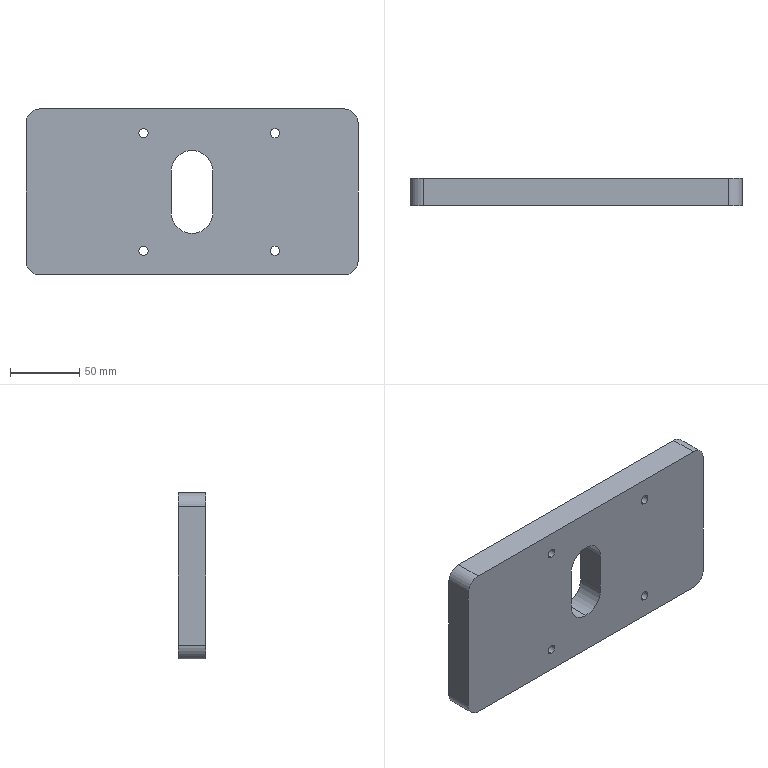Part | SolidWorks | features BaseBody 1 | 1 solid | 23 faces | box 240 x 20 x 120 mm | volume 539241 mm3 | cylinder 15 | plane 8 | commonest cylinder face diameters 6.8 x8 20 x4 30 x3
STEP:
#1=CARTESIAN_POINT('',(-35.,-10.,-45.9));
#2=VERTEX_POINT('',#1);
#3=CARTESIAN_POINT('',(-35.,-10.,-39.1));
#4=VERTEX_POINT('',#3);
#5=CARTESIAN_POINT('',(-35.,-10.,-42.5));
#6=DIRECTION('',(0.,1.,0.));
#7=DIRECTION('',(0.,0.,1.));
#8=AXIS2_PLACEMENT_3D('',#5,#6,#7);
#9=CIRCLE('',#8,3.4);
#10=EDGE_CURVE('',#2,#4,#9,.T.);
#11=ORIENTED_EDGE('',*,*,#10,.F.);
#12=CARTESIAN_POINT('',(-35.,10.,-45.9));
#13=VERTEX_POINT('',#12);
#14=CARTESIAN_POINT('',(-35.,10.,-45.9));
#15=DIRECTION('',(0.,1.,0.));
#16=VECTOR('',#15,1000.);
#17=LINE('',#14,#16);
#18=EDGE_CURVE('',#2,#13,#17,.T.);
#19=ORIENTED_EDGE('',*,*,#18,.T.);
#20=CARTESIAN_POINT('',(-35.,10.,-39.1));
#21=VERTEX_POINT('',#20);
#22=CARTESIAN_POINT('',(-35.,10.,-42.5));
#23=DIRECTION('',(0.,1.,0.));
#24=DIRECTION('',(0.,0.,1.));
#25=AXIS2_PLACEMENT_3D('',#22,#23,#24);
#26=CIRCLE('',#25,3.4);
#27=EDGE_CURVE('',#13,#21,#26,.T.);
#28=ORIENTED_EDGE('',*,*,#27,.T.);
#29=CARTESIAN_POINT('',(-35.,10.,-39.1));
#30=DIRECTION('',(0.,1.,0.));
#31=VECTOR('',#30,1000.);
#32=LINE('',#29,#31);
#33=EDGE_CURVE('',#4,#21,#32,.T.);
#34=ORIENTED_EDGE('',*,*,#33,.F.);
#35=EDGE_LOOP('',(#11,#19,#28,#34));
#36=FACE_OUTER_BOUND('',#35,.T.);
#37=CARTESIAN_POINT('',(-35.,10.,-42.5));
#38=DIRECTION('',(0.,1.,0.));
#39=DIRECTION('',(0.,0.,1.));
#40=AXIS2_PLACEMENT_3D('',#37,#38,#39);
#41=CYLINDRICAL_SURFACE('',#40,3.4);
#42=ADVANCED_FACE('',(#36),#41,.F.);
#43=CARTESIAN_POINT('',(60.,-10.,-45.9));
#44=VERTEX_POINT('',#43);
#45=CARTESIAN_POINT('',(60.,-10.,-39.1));
#46=VERTEX_POINT('',#45);
#47=CARTESIAN_POINT('',(60.,-10.,-42.5));
#48=DIRECTION('',(0.,1.,0.));
#49=DIRECTION('',(0.,0.,1.));
#50=AXIS2_PLACEMENT_3D('',#47,#48,#49);
#51=CIRCLE('',#50,3.4);
#52=EDGE_CURVE('',#44,#46,#51,.T.);
#53=ORIENTED_EDGE('',*,*,#52,.F.);
#54=CARTESIAN_POINT('',(60.,10.,-45.9));
#55=VERTEX_POINT('',#54);
#56=CARTESIAN_POINT('',(60.,10.,-45.9));
#57=DIRECTION('',(0.,1.,0.));
#58=VECTOR('',#57,1000.);
#59=LINE('',#56,#58);
#60=EDGE_CURVE('',#44,#55,#59,.T.);
#61=ORIENTED_EDGE('',*,*,#60,.T.);
#62=CARTESIAN_POINT('',(60.,10.,-39.1));
#63=VERTEX_POINT('',#62);
#64=CARTESIAN_POINT('',(60.,10.,-42.5));
#65=DIRECTION('',(0.,1.,0.));
#66=DIRECTION('',(0.,0.,1.));
#67=AXIS2_PLACEMENT_3D('',#64,#65,#66);
#68=CIRCLE('',#67,3.4);
#69=EDGE_CURVE('',#55,#63,#68,.T.);
#70=ORIENTED_EDGE('',*,*,#69,.T.);
#71=CARTESIAN_POINT('',(60.,10.,-39.1));
#72=DIRECTION('',(0.,1.,0.));
#73=VECTOR('',#72,1000.);
#74=LINE('',#71,#73);
#75=EDGE_CURVE('',#46,#63,#74,.T.);
#76=ORIENTED_EDGE('',*,*,#75,.F.);
#77=EDGE_LOOP('',(#53,#61,#70,#76));
#78=FACE_OUTER_BOUND('',#77,.T.);
#79=CARTESIAN_POINT('',(60.,10.,-42.5));
#80=DIRECTION('',(0.,1.,0.));
#81=DIRECTION('',(0.,0.,1.));
#82=AXIS2_PLACEMENT_3D('',#79,#80,#81);
#83=CYLINDRICAL_SURFACE('',#82,3.4);
#84=ADVANCED_FACE('',(#78),#83,.F.);
#85=CARTESIAN_POINT('',(60.,-10.,39.1));
#86=VERTEX_POINT('',#85);
#87=CARTESIAN_POINT('',(60.,-10.,45.9));
#88=VERTEX_POINT('',#87);
#89=CARTESIAN_POINT('',(60.,-10.,42.5));
#90=DIRECTION('',(0.,1.,0.));
#91=DIRECTION('',(0.,0.,1.));
#92=AXIS2_PLACEMENT_3D('',#89,#90,#91);
#93=CIRCLE('',#92,3.4);
#94=EDGE_CURVE('',#86,#88,#93,.T.);
#95=ORIENTED_EDGE('',*,*,#94,.F.);
#96=CARTESIAN_POINT('',(60.,10.,39.1));
#97=VERTEX_POINT('',#96);
#98=CARTESIAN_POINT('',(60.,10.,39.1));
#99=DIRECTION('',(0.,1.,0.));
#100=VECTOR('',#99,1000.);
#101=LINE('',#98,#100);
#102=EDGE_CURVE('',#86,#97,#101,.T.);
#103=ORIENTED_EDGE('',*,*,#102,.T.);
#104=CARTESIAN_POINT('',(60.,10.,45.9));
#105=VERTEX_POINT('',#104);
#106=CARTESIAN_POINT('',(60.,10.,42.5));
#107=DIRECTION('',(0.,1.,0.));
#108=DIRECTION('',(0.,0.,1.));
#109=AXIS2_PLACEMENT_3D('',#106,#107,#108);
#110=CIRCLE('',#109,3.4);
#111=EDGE_CURVE('',#97,#105,#110,.T.);
#112=ORIENTED_EDGE('',*,*,#111,.T.);
#113=CARTESIAN_POINT('',(60.,10.,45.9));
#114=DIRECTION('',(0.,1.,0.));
#115=VECTOR('',#114,1000.);
#116=LINE('',#113,#115);
#117=EDGE_CURVE('',#88,#105,#116,.T.);
#118=ORIENTED_EDGE('',*,*,#117,.F.);
#119=EDGE_LOOP('',(#95,#103,#112,#118));
#120=FACE_OUTER_BOUND('',#119,.T.);
#121=CARTESIAN_POINT('',(60.,10.,42.5));
#122=DIRECTION('',(0.,1.,0.));
#123=DIRECTION('',(0.,0.,1.));
#124=AXIS2_PLACEMENT_3D('',#121,#122,#123);
#125=CYLINDRICAL_SURFACE('',#124,3.4);
#126=ADVANCED_FACE('',(#120),#125,.F.);
#127=CARTESIAN_POINT('',(-35.,-10.,39.1));
#128=VERTEX_POINT('',#127);
#129=CARTESIAN_POINT('',(-35.,-10.,45.9));
#130=VERTEX_POINT('',#129);
#131=CARTESIAN_POINT('',(-35.,-10.,42.5));
#132=DIRECTION('',(0.,1.,0.));
#133=DIRECTION('',(0.,0.,1.));
#134=AXIS2_PLACEMENT_3D('',#131,#132,#133);
#135=CIRCLE('',#134,3.4);
#136=EDGE_CURVE('',#128,#130,#135,.T.);
#137=ORIENTED_EDGE('',*,*,#136,.F.);
#138=CARTESIAN_POINT('',(-35.,10.,39.1));
#139=VERTEX_POINT('',#138);
#140=CARTESIAN_POINT('',(-35.,10.,39.1));
#141=DIRECTION('',(0.,1.,0.));
#142=VECTOR('',#141,1000.);
#143=LINE('',#140,#142);
#144=EDGE_CURVE('',#128,#139,#143,.T.);
#145=ORIENTED_EDGE('',*,*,#144,.T.);
#146=CARTESIAN_POINT('',(-35.,10.,45.9));
#147=VERTEX_POINT('',#146);
#148=CARTESIAN_POINT('',(-35.,10.,42.5));
#149=DIRECTION('',(0.,1.,0.));
#150=DIRECTION('',(0.,0.,1.));
#151=AXIS2_PLACEMENT_3D('',#148,#149,#150);
#152=CIRCLE('',#151,3.4);
#153=EDGE_CURVE('',#139,#147,#152,.T.);
#154=ORIENTED_EDGE('',*,*,#153,.T.);
#155=CARTESIAN_POINT('',(-35.,10.,45.9));
#156=DIRECTION('',(0.,1.,0.));
#157=VECTOR('',#156,1000.);
#158=LINE('',#155,#157);
#159=EDGE_CURVE('',#130,#147,#158,.T.);
#160=ORIENTED_EDGE('',*,*,#159,.F.);
#161=EDGE_LOOP('',(#137,#145,#154,#160));
#162=FACE_OUTER_BOUND('',#161,.T.);
#163=CARTESIAN_POINT('',(-35.,10.,42.5));
#164=DIRECTION('',(0.,1.,0.));
#165=DIRECTION('',(0.,0.,1.));
#166=AXIS2_PLACEMENT_3D('',#163,#164,#165);
#167=CYLINDRICAL_SURFACE('',#166,3.4);
#168=ADVANCED_FACE('',(#162),#167,.F.);
#169=CARTESIAN_POINT('',(15.,10.,-15.));
#170=VERTEX_POINT('',#169);
#171=CARTESIAN_POINT('',(0.,10.,-30.));
#172=VERTEX_POINT('',#171);
#173=CARTESIAN_POINT('',(0.,10.,-15.));
#174=DIRECTION('',(0.,1.,0.));
#175=DIRECTION('',(0.,0.,1.));
#176=AXIS2_PLACEMENT_3D('',#173,#174,#175);
#177=CIRCLE('',#176,15.);
#178=EDGE_CURVE('',#170,#172,#177,.T.);
#179=ORIENTED_EDGE('',*,*,#178,.T.);
#180=CARTESIAN_POINT('',(0.,-10.,-30.));
#181=VERTEX_POINT('',#180);
#182=CARTESIAN_POINT('',(0.,10.,-30.));
#183=DIRECTION('',(0.,-1.,0.));
#184=VECTOR('',#183,1000.);
#185=LINE('',#182,#184);
#186=EDGE_CURVE('',#172,#181,#185,.T.);
#187=ORIENTED_EDGE('',*,*,#186,.T.);
#188=CARTESIAN_POINT('',(15.,-10.,-15.));
#189=VERTEX_POINT('',#188);
#190=CARTESIAN_POINT('',(0.,-10.,-15.));
#191=DIRECTION('',(0.,1.,0.));
#192=DIRECTION('',(0.,0.,1.));
#193=AXIS2_PLACEMENT_3D('',#190,#191,#192);
#194=CIRCLE('',#193,15.);
#195=EDGE_CURVE('',#189,#181,#194,.T.);
#196=ORIENTED_EDGE('',*,*,#195,.F.);
#197=CARTESIAN_POINT('',(15.,10.,-15.));
#198=DIRECTION('',(0.,-1.,0.));
#199=VECTOR('',#198,1000.);
#200=LINE('',#197,#199);
#201=EDGE_CURVE('',#170,#189,#200,.T.);
#202=ORIENTED_EDGE('',*,*,#201,.F.);
#203=EDGE_LOOP('',(#179,#187,#196,#202));
#204=FACE_OUTER_BOUND('',#203,.T.);
#205=CARTESIAN_POINT('',(0.,10.,-15.));
#206=DIRECTION('',(0.,-1.,0.));
#207=DIRECTION('',(0.,0.,-1.));
#208=AXIS2_PLACEMENT_3D('',#205,#206,#207);
#209=CYLINDRICAL_SURFACE('',#208,15.);
#210=ADVANCED_FACE('',(#204),#209,.F.);
#211=CARTESIAN_POINT('',(-35.,10.,-42.5));
#212=DIRECTION('',(0.,1.,0.));
#213=DIRECTION('',(0.,0.,1.));
#214=AXIS2_PLACEMENT_3D('',#211,#212,#213);
#215=CIRCLE('',#214,3.4);
#216=EDGE_CURVE('',#21,#13,#215,.T.);
#217=ORIENTED_EDGE('',*,*,#216,.F.);
#218=ORIENTED_EDGE('',*,*,#27,.F.);
#219=EDGE_LOOP('',(#217,#218));
#220=FACE_BOUND('',#219,.T.);
#221=CARTESIAN_POINT('',(60.,10.,-42.5));
#222=DIRECTION('',(0.,1.,0.));
#223=DIRECTION('',(0.,0.,1.));
#224=AXIS2_PLACEMENT_3D('',#221,#222,#223);
#225=CIRCLE('',#224,3.4);
#226=EDGE_CURVE('',#63,#55,#225,.T.);
#227=ORIENTED_EDGE('',*,*,#226,.F.);
#228=ORIENTED_EDGE('',*,*,#69,.F.);
#229=EDGE_LOOP('',(#227,#228));
#230=FACE_BOUND('',#229,.T.);
#231=CARTESIAN_POINT('',(60.,10.,42.5));
#232=DIRECTION('',(0.,1.,0.));
#233=DIRECTION('',(0.,0.,1.));
#234=AXIS2_PLACEMENT_3D('',#231,#232,#233);
#235=CIRCLE('',#234,3.4);
#236=EDGE_CURVE('',#105,#97,#235,.T.);
#237=ORIENTED_EDGE('',*,*,#236,.F.);
#238=ORIENTED_EDGE('',*,*,#111,.F.);
#239=EDGE_LOOP('',(#237,#238));
#240=FACE_BOUND('',#239,.T.);
#241=CARTESIAN_POINT('',(-35.,10.,42.5));
#242=DIRECTION('',(0.,1.,0.));
#243=DIRECTION('',(0.,0.,1.));
#244=AXIS2_PLACEMENT_3D('',#241,#242,#243);
#245=CIRCLE('',#244,3.4);
#246=EDGE_CURVE('',#147,#139,#245,.T.);
#247=ORIENTED_EDGE('',*,*,#246,.F.);
#248=ORIENTED_EDGE('',*,*,#153,.F.);
#249=EDGE_LOOP('',(#247,#248));
#250=FACE_BOUND('',#249,.T.);
#251=CARTESIAN_POINT('',(110.,10.,60.));
#252=VERTEX_POINT('',#251);
#253=CARTESIAN_POINT('',(120.,10.,50.));
#254=VERTEX_POINT('',#253);
#255=CARTESIAN_POINT('',(110.,10.,50.));
#256=DIRECTION('',(0.,1.,0.));
#257=DIRECTION('',(0.,0.,1.));
#258=AXIS2_PLACEMENT_3D('',#255,#256,#257);
#259=CIRCLE('',#258,10.);
#260=EDGE_CURVE('',#252,#254,#259,.T.);
#261=ORIENTED_EDGE('',*,*,#260,.T.);
#262=CARTESIAN_POINT('',(120.,10.,-50.));
#263=VERTEX_POINT('',#262);
#264=CARTESIAN_POINT('',(120.,10.,-50.));
#265=DIRECTION('',(0.,0.,-1.));
#266=VECTOR('',#265,1000.);
#267=LINE('',#264,#266);
#268=EDGE_CURVE('',#254,#263,#267,.T.);
#269=ORIENTED_EDGE('',*,*,#268,.T.);
#270=CARTESIAN_POINT('',(110.,10.,-60.));
#271=VERTEX_POINT('',#270);
#272=CARTESIAN_POINT('',(110.,10.,-50.));
#273=DIRECTION('',(0.,1.,0.));
#274=DIRECTION('',(0.,0.,-1.));
#275=AXIS2_PLACEMENT_3D('',#272,#273,#274);
#276=CIRCLE('',#275,10.);
#277=EDGE_CURVE('',#263,#271,#276,.T.);
#278=ORIENTED_EDGE('',*,*,#277,.T.);
#279=CARTESIAN_POINT('',(-110.,10.,-60.));
#280=VERTEX_POINT('',#279);
#281=CARTESIAN_POINT('',(-110.,10.,-60.));
#282=DIRECTION('',(-1.,0.,0.));
#283=VECTOR('',#282,1000.);
#284=LINE('',#281,#283);
#285=EDGE_CURVE('',#271,#280,#284,.T.);
#286=ORIENTED_EDGE('',*,*,#285,.T.);
#287=CARTESIAN_POINT('',(-120.,10.,-50.));
#288=VERTEX_POINT('',#287);
#289=CARTESIAN_POINT('',(-110.,10.,-50.));
#290=DIRECTION('',(0.,1.,0.));
#291=DIRECTION('',(0.,0.,1.));
#292=AXIS2_PLACEMENT_3D('',#289,#290,#291);
#293=CIRCLE('',#292,10.);
#294=EDGE_CURVE('',#280,#288,#293,.T.);
#295=ORIENTED_EDGE('',*,*,#294,.T.);
#296=CARTESIAN_POINT('',(-120.,10.,50.));
#297=VERTEX_POINT('',#296);
#298=CARTESIAN_POINT('',(-120.,10.,-50.));
#299=DIRECTION('',(0.,0.,1.));
#300=VECTOR('',#299,1000.);
#301=LINE('',#298,#300);
#302=EDGE_CURVE('',#288,#297,#301,.T.);
#303=ORIENTED_EDGE('',*,*,#302,.T.);
#304=CARTESIAN_POINT('',(-110.,10.,60.));
#305=VERTEX_POINT('',#304);
#306=CARTESIAN_POINT('',(-110.,10.,50.));
#307=DIRECTION('',(0.,1.,0.));
#308=DIRECTION('',(0.,0.,1.));
#309=AXIS2_PLACEMENT_3D('',#306,#307,#308);
#310=CIRCLE('',#309,10.);
#311=EDGE_CURVE('',#297,#305,#310,.T.);
#312=ORIENTED_EDGE('',*,*,#311,.T.);
#313=CARTESIAN_POINT('',(-110.,10.,60.));
#314=DIRECTION('',(1.,0.,0.));
#315=VECTOR('',#314,1000.);
#316=LINE('',#313,#315);
#317=EDGE_CURVE('',#305,#252,#316,.T.);
#318=ORIENTED_EDGE('',*,*,#317,.T.);
#319=EDGE_LOOP('',(#261,#269,#278,#286,#295,#303,#312,#318));
#320=FACE_OUTER_BOUND('',#319,.T.);
#321=CARTESIAN_POINT('',(-15.,10.,-15.));
#322=VERTEX_POINT('',#321);
#323=CARTESIAN_POINT('',(-15.,10.,15.));
#324=VERTEX_POINT('',#323);
#325=CARTESIAN_POINT('',(-15.,10.,-15.));
#326=DIRECTION('',(0.,0.,1.));
#327=VECTOR('',#326,1000.);
#328=LINE('',#325,#327);
#329=EDGE_CURVE('',#322,#324,#328,.T.);
#330=ORIENTED_EDGE('',*,*,#329,.F.);
#331=CARTESIAN_POINT('',(0.,10.,-15.));
#332=DIRECTION('',(0.,1.,0.));
#333=DIRECTION('',(0.,0.,1.));
#334=AXIS2_PLACEMENT_3D('',#331,#332,#333);
#335=CIRCLE('',#334,15.);
#336=EDGE_CURVE('',#172,#322,#335,.T.);
#337=ORIENTED_EDGE('',*,*,#336,.F.);
#338=ORIENTED_EDGE('',*,*,#178,.F.);
#339=CARTESIAN_POINT('',(15.,10.,15.));
#340=VERTEX_POINT('',#339);
#341=CARTESIAN_POINT('',(15.,10.,-15.));
#342=DIRECTION('',(0.,0.,-1.));
#343=VECTOR('',#342,1000.);
#344=LINE('',#341,#343);
#345=EDGE_CURVE('',#340,#170,#344,.T.);
#346=ORIENTED_EDGE('',*,*,#345,.F.);
#347=CARTESIAN_POINT('',(0.,10.,15.));
#348=DIRECTION('',(0.,1.,0.));
#349=DIRECTION('',(0.,0.,1.));
#350=AXIS2_PLACEMENT_3D('',#347,#348,#349);
#351=CIRCLE('',#350,15.);
#352=EDGE_CURVE('',#324,#340,#351,.T.);
#353=ORIENTED_EDGE('',*,*,#352,.F.);
#354=EDGE_LOOP('',(#330,#337,#338,#346,#353));
#355=FACE_BOUND('',#354,.T.);
#356=CARTESIAN_POINT('',(110.,10.,50.));
#357=DIRECTION('',(0.,1.,0.));
#358=DIRECTION('',(0.,0.,1.));
#359=AXIS2_PLACEMENT_3D('',#356,#357,#358);
#360=PLANE('',#359);
#361=ADVANCED_FACE('',(#220,#230,#240,#250,#320,#355),#360,.T.);
#362=CARTESIAN_POINT('',(-35.,-10.,-42.5));
#363=DIRECTION('',(0.,1.,0.));
#364=DIRECTION('',(0.,0.,1.));
#365=AXIS2_PLACEMENT_3D('',#362,#363,#364);
#366=CIRCLE('',#365,3.4);
#367=EDGE_CURVE('',#4,#2,#366,.T.);
#368=ORIENTED_EDGE('',*,*,#367,.T.);
#369=ORIENTED_EDGE('',*,*,#10,.T.);
#370=EDGE_LOOP('',(#368,#369));
#371=FACE_BOUND('',#370,.T.);
#372=CARTESIAN_POINT('',(60.,-10.,-42.5));
#373=DIRECTION('',(0.,1.,0.));
#374=DIRECTION('',(0.,0.,1.));
#375=AXIS2_PLACEMENT_3D('',#372,#373,#374);
#376=CIRCLE('',#375,3.4);
#377=EDGE_CURVE('',#46,#44,#376,.T.);
#378=ORIENTED_EDGE('',*,*,#377,.T.);
#379=ORIENTED_EDGE('',*,*,#52,.T.);
#380=EDGE_LOOP('',(#378,#379));
#381=FACE_BOUND('',#380,.T.);
#382=CARTESIAN_POINT('',(60.,-10.,42.5));
#383=DIRECTION('',(0.,1.,0.));
#384=DIRECTION('',(0.,0.,1.));
#385=AXIS2_PLACEMENT_3D('',#382,#383,#384);
#386=CIRCLE('',#385,3.4);
#387=EDGE_CURVE('',#88,#86,#386,.T.);
#388=ORIENTED_EDGE('',*,*,#387,.T.);
#389=ORIENTED_EDGE('',*,*,#94,.T.);
#390=EDGE_LOOP('',(#388,#389));
#391=FACE_BOUND('',#390,.T.);
#392=CARTESIAN_POINT('',(-35.,-10.,42.5));
#393=DIRECTION('',(0.,1.,0.));
#394=DIRECTION('',(0.,0.,1.));
#395=AXIS2_PLACEMENT_3D('',#392,#393,#394);
#396=CIRCLE('',#395,3.4);
#397=EDGE_CURVE('',#130,#128,#396,.T.);
#398=ORIENTED_EDGE('',*,*,#397,.T.);
#399=ORIENTED_EDGE('',*,*,#136,.T.);
#400=EDGE_LOOP('',(#398,#399));
#401=FACE_BOUND('',#400,.T.);
#402=CARTESIAN_POINT('',(110.,-10.,60.));
#403=VERTEX_POINT('',#402);
#404=CARTESIAN_POINT('',(120.,-10.,50.));
#405=VERTEX_POINT('',#404);
#406=CARTESIAN_POINT('',(110.,-10.,50.));
#407=DIRECTION('',(0.,1.,0.));
#408=DIRECTION('',(0.,0.,1.));
#409=AXIS2_PLACEMENT_3D('',#406,#407,#408);
#410=CIRCLE('',#409,10.);
#411=EDGE_CURVE('',#403,#405,#410,.T.);
#412=ORIENTED_EDGE('',*,*,#411,.F.);
#413=CARTESIAN_POINT('',(-110.,-10.,60.));
#414=VERTEX_POINT('',#413);
#415=CARTESIAN_POINT('',(-110.,-10.,60.));
#416=DIRECTION('',(1.,0.,0.));
#417=VECTOR('',#416,1000.);
#418=LINE('',#415,#417);
#419=EDGE_CURVE('',#414,#403,#418,.T.);
#420=ORIENTED_EDGE('',*,*,#419,.F.);
#421=CARTESIAN_POINT('',(-120.,-10.,50.));
#422=VERTEX_POINT('',#421);
#423=CARTESIAN_POINT('',(-110.,-10.,50.));
#424=DIRECTION('',(0.,1.,0.));
#425=DIRECTION('',(0.,0.,1.));
#426=AXIS2_PLACEMENT_3D('',#423,#424,#425);
#427=CIRCLE('',#426,10.);
#428=EDGE_CURVE('',#422,#414,#427,.T.);
#429=ORIENTED_EDGE('',*,*,#428,.F.);
#430=CARTESIAN_POINT('',(-120.,-10.,-50.));
#431=VERTEX_POINT('',#430);
#432=CARTESIAN_POINT('',(-120.,-10.,-50.));
#433=DIRECTION('',(0.,0.,1.));
#434=VECTOR('',#433,1000.);
#435=LINE('',#432,#434);
#436=EDGE_CURVE('',#431,#422,#435,.T.);
#437=ORIENTED_EDGE('',*,*,#436,.F.);
#438=CARTESIAN_POINT('',(-110.,-10.,-60.));
#439=VERTEX_POINT('',#438);
#440=CARTESIAN_POINT('',(-110.,-10.,-50.));
#441=DIRECTION('',(0.,1.,0.));
#442=DIRECTION('',(0.,0.,1.));
#443=AXIS2_PLACEMENT_3D('',#440,#441,#442);
#444=CIRCLE('',#443,10.);
#445=EDGE_CURVE('',#439,#431,#444,.T.);
#446=ORIENTED_EDGE('',*,*,#445,.F.);
#447=CARTESIAN_POINT('',(110.,-10.,-60.));
#448=VERTEX_POINT('',#447);
#449=CARTESIAN_POINT('',(-110.,-10.,-60.));
#450=DIRECTION('',(-1.,0.,0.));
#451=VECTOR('',#450,1000.);
#452=LINE('',#449,#451);
#453=EDGE_CURVE('',#448,#439,#452,.T.);
#454=ORIENTED_EDGE('',*,*,#453,.F.);
#455=CARTESIAN_POINT('',(120.,-10.,-50.));
#456=VERTEX_POINT('',#455);
#457=CARTESIAN_POINT('',(110.,-10.,-50.));
#458=DIRECTION('',(0.,1.,0.));
#459=DIRECTION('',(0.,0.,-1.));
#460=AXIS2_PLACEMENT_3D('',#457,#458,#459);
#461=CIRCLE('',#460,10.);
#462=EDGE_CURVE('',#456,#448,#461,.T.);
#463=ORIENTED_EDGE('',*,*,#462,.F.);
#464=CARTESIAN_POINT('',(120.,-10.,-50.));
#465=DIRECTION('',(0.,0.,-1.));
#466=VECTOR('',#465,1000.);
#467=LINE('',#464,#466);
#468=EDGE_CURVE('',#405,#456,#467,.T.);
#469=ORIENTED_EDGE('',*,*,#468,.F.);
#470=EDGE_LOOP('',(#412,#420,#429,#437,#446,#454,#463,#469));
#471=FACE_OUTER_BOUND('',#470,.T.);
#472=ORIENTED_EDGE('',*,*,#195,.T.);
#473=CARTESIAN_POINT('',(-15.,-10.,-15.));
#474=VERTEX_POINT('',#473);
#475=CARTESIAN_POINT('',(0.,-10.,-15.));
#476=DIRECTION('',(0.,1.,0.));
#477=DIRECTION('',(0.,0.,1.));
#478=AXIS2_PLACEMENT_3D('',#475,#476,#477);
#479=CIRCLE('',#478,15.);
#480=EDGE_CURVE('',#181,#474,#479,.T.);
#481=ORIENTED_EDGE('',*,*,#480,.T.);
#482=CARTESIAN_POINT('',(-15.,-10.,15.));
#483=VERTEX_POINT('',#482);
#484=CARTESIAN_POINT('',(-15.,-10.,-15.));
#485=DIRECTION('',(0.,0.,1.));
#486=VECTOR('',#485,1000.);
#487=LINE('',#484,#486);
#488=EDGE_CURVE('',#474,#483,#487,.T.);
#489=ORIENTED_EDGE('',*,*,#488,.T.);
#490=CARTESIAN_POINT('',(15.,-10.,15.));
#491=VERTEX_POINT('',#490);
#492=CARTESIAN_POINT('',(0.,-10.,15.));
#493=DIRECTION('',(0.,1.,0.));
#494=DIRECTION('',(0.,0.,1.));
#495=AXIS2_PLACEMENT_3D('',#492,#493,#494);
#496=CIRCLE('',#495,15.);
#497=EDGE_CURVE('',#483,#491,#496,.T.);
#498=ORIENTED_EDGE('',*,*,#497,.T.);
#499=CARTESIAN_POINT('',(15.,-10.,-15.));
#500=DIRECTION('',(0.,0.,-1.));
#501=VECTOR('',#500,1000.);
#502=LINE('',#499,#501);
#503=EDGE_CURVE('',#491,#189,#502,.T.);
#504=ORIENTED_EDGE('',*,*,#503,.T.);
#505=EDGE_LOOP('',(#472,#481,#489,#498,#504));
#506=FACE_BOUND('',#505,.T.);
#507=CARTESIAN_POINT('',(110.,-10.,50.));
#508=DIRECTION('',(0.,1.,0.));
#509=DIRECTION('',(0.,0.,1.));
#510=AXIS2_PLACEMENT_3D('',#507,#508,#509);
#511=PLANE('',#510);
#512=ADVANCED_FACE('',(#371,#381,#391,#401,#471,#506),#511,.F.);
#513=ORIENTED_EDGE('',*,*,#411,.T.);
#514=CARTESIAN_POINT('',(120.,10.,50.));
#515=DIRECTION('',(0.,-1.,0.));
#516=VECTOR('',#515,1000.);
#517=LINE('',#514,#516);
#518=EDGE_CURVE('',#254,#405,#517,.T.);
#519=ORIENTED_EDGE('',*,*,#518,.F.);
#520=ORIENTED_EDGE('',*,*,#260,.F.);
#521=CARTESIAN_POINT('',(110.,10.,60.));
#522=DIRECTION('',(0.,-1.,0.));
#523=VECTOR('',#522,1000.);
#524=LINE('',#521,#523);
#525=EDGE_CURVE('',#252,#403,#524,.T.);
#526=ORIENTED_EDGE('',*,*,#525,.T.);
#527=EDGE_LOOP('',(#513,#519,#520,#526));
#528=FACE_OUTER_BOUND('',#527,.T.);
#529=CARTESIAN_POINT('',(110.,10.,50.));
#530=DIRECTION('',(0.,-1.,0.));
#531=DIRECTION('',(0.,0.,-1.));
#532=AXIS2_PLACEMENT_3D('',#529,#530,#531);
#533=CYLINDRICAL_SURFACE('',#532,10.);
#534=ADVANCED_FACE('',(#528),#533,.T.);
#535=ORIENTED_EDGE('',*,*,#468,.T.);
#536=CARTESIAN_POINT('',(120.,10.,-50.));
#537=DIRECTION('',(0.,-1.,0.));
#538=VECTOR('',#537,1000.);
#539=LINE('',#536,#538);
#540=EDGE_CURVE('',#263,#456,#539,.T.);
#541=ORIENTED_EDGE('',*,*,#540,.F.);
#542=ORIENTED_EDGE('',*,*,#268,.F.);
#543=ORIENTED_EDGE('',*,*,#518,.T.);
#544=EDGE_LOOP('',(#535,#541,#542,#543));
#545=FACE_OUTER_BOUND('',#544,.T.);
#546=CARTESIAN_POINT('',(120.,10.,-50.));
#547=DIRECTION('',(-1.,0.,0.));
#548=DIRECTION('',(0.,0.,1.));
#549=AXIS2_PLACEMENT_3D('',#546,#547,#548);
#550=PLANE('',#549);
#551=ADVANCED_FACE('',(#545),#550,.F.);
#552=ORIENTED_EDGE('',*,*,#462,.T.);
#553=CARTESIAN_POINT('',(110.,10.,-60.));
#554=DIRECTION('',(0.,-1.,0.));
#555=VECTOR('',#554,1000.);
#556=LINE('',#553,#555);
#557=EDGE_CURVE('',#271,#448,#556,.T.);
#558=ORIENTED_EDGE('',*,*,#557,.F.);
#559=ORIENTED_EDGE('',*,*,#277,.F.);
#560=ORIENTED_EDGE('',*,*,#540,.T.);
#561=EDGE_LOOP('',(#552,#558,#559,#560));
#562=FACE_OUTER_BOUND('',#561,.T.);
#563=CARTESIAN_POINT('',(110.,10.,-50.));
#564=DIRECTION('',(0.,-1.,0.));
#565=DIRECTION('',(0.,0.,-1.));
#566=AXIS2_PLACEMENT_3D('',#563,#564,#565);
#567=CYLINDRICAL_SURFACE('',#566,10.);
#568=ADVANCED_FACE('',(#562),#567,.T.);
#569=ORIENTED_EDGE('',*,*,#453,.T.);
#570=CARTESIAN_POINT('',(-110.,10.,-60.));
#571=DIRECTION('',(0.,-1.,0.));
#572=VECTOR('',#571,1000.);
#573=LINE('',#570,#572);
#574=EDGE_CURVE('',#280,#439,#573,.T.);
#575=ORIENTED_EDGE('',*,*,#574,.F.);
#576=ORIENTED_EDGE('',*,*,#285,.F.);
#577=ORIENTED_EDGE('',*,*,#557,.T.);
#578=EDGE_LOOP('',(#569,#575,#576,#577));
#579=FACE_OUTER_BOUND('',#578,.T.);
#580=CARTESIAN_POINT('',(-110.,10.,-60.));
#581=DIRECTION('',(0.,0.,1.));
#582=DIRECTION('',(1.,0.,0.));
#583=AXIS2_PLACEMENT_3D('',#580,#581,#582);
#584=PLANE('',#583);
#585=ADVANCED_FACE('',(#579),#584,.F.);
#586=ORIENTED_EDGE('',*,*,#445,.T.);
#587=CARTESIAN_POINT('',(-120.,10.,-50.));
#588=DIRECTION('',(0.,-1.,0.));
#589=VECTOR('',#588,1000.);
#590=LINE('',#587,#589);
#591=EDGE_CURVE('',#288,#431,#590,.T.);
#592=ORIENTED_EDGE('',*,*,#591,.F.);
#593=ORIENTED_EDGE('',*,*,#294,.F.);
#594=ORIENTED_EDGE('',*,*,#574,.T.);
#595=EDGE_LOOP('',(#586,#592,#593,#594));
#596=FACE_OUTER_BOUND('',#595,.T.);
#597=CARTESIAN_POINT('',(-110.,10.,-50.));
#598=DIRECTION('',(0.,-1.,0.));
#599=DIRECTION('',(0.,0.,-1.));
#600=AXIS2_PLACEMENT_3D('',#597,#598,#599);
#601=CYLINDRICAL_SURFACE('',#600,10.);
#602=ADVANCED_FACE('',(#596),#601,.T.);
#603=ORIENTED_EDGE('',*,*,#436,.T.);
#604=CARTESIAN_POINT('',(-120.,10.,50.));
#605=DIRECTION('',(0.,-1.,0.));
#606=VECTOR('',#605,1000.);
#607=LINE('',#604,#606);
#608=EDGE_CURVE('',#297,#422,#607,.T.);
#609=ORIENTED_EDGE('',*,*,#608,.F.);
#610=ORIENTED_EDGE('',*,*,#302,.F.);
#611=ORIENTED_EDGE('',*,*,#591,.T.);
#612=EDGE_LOOP('',(#603,#609,#610,#611));
#613=FACE_OUTER_BOUND('',#612,.T.);
#614=CARTESIAN_POINT('',(-120.,10.,-50.));
#615=DIRECTION('',(1.,0.,0.));
#616=DIRECTION('',(0.,0.,-1.));
#617=AXIS2_PLACEMENT_3D('',#614,#615,#616);
#618=PLANE('',#617);
#619=ADVANCED_FACE('',(#613),#618,.F.);
#620=ORIENTED_EDGE('',*,*,#428,.T.);
#621=CARTESIAN_POINT('',(-110.,10.,60.));
#622=DIRECTION('',(0.,-1.,0.));
#623=VECTOR('',#622,1000.);
#624=LINE('',#621,#623);
#625=EDGE_CURVE('',#305,#414,#624,.T.);
#626=ORIENTED_EDGE('',*,*,#625,.F.);
#627=ORIENTED_EDGE('',*,*,#311,.F.);
#628=ORIENTED_EDGE('',*,*,#608,.T.);
#629=EDGE_LOOP('',(#620,#626,#627,#628));
#630=FACE_OUTER_BOUND('',#629,.T.);
#631=CARTESIAN_POINT('',(-110.,10.,50.));
#632=DIRECTION('',(0.,-1.,0.));
#633=DIRECTION('',(0.,0.,-1.));
#634=AXIS2_PLACEMENT_3D('',#631,#632,#633);
#635=CYLINDRICAL_SURFACE('',#634,10.);
#636=ADVANCED_FACE('',(#630),#635,.T.);
#637=ORIENTED_EDGE('',*,*,#419,.T.);
#638=ORIENTED_EDGE('',*,*,#525,.F.);
#639=ORIENTED_EDGE('',*,*,#317,.F.);
#640=ORIENTED_EDGE('',*,*,#625,.T.);
#641=EDGE_LOOP('',(#637,#638,#639,#640));
#642=FACE_OUTER_BOUND('',#641,.T.);
#643=CARTESIAN_POINT('',(-110.,10.,60.));
#644=DIRECTION('',(0.,0.,-1.));
#645=DIRECTION('',(-1.,0.,0.));
#646=AXIS2_PLACEMENT_3D('',#643,#644,#645);
#647=PLANE('',#646);
#648=ADVANCED_FACE('',(#642),#647,.F.);
#649=ORIENTED_EDGE('',*,*,#186,.F.);
#650=ORIENTED_EDGE('',*,*,#336,.T.);
#651=CARTESIAN_POINT('',(-15.,10.,-15.));
#652=DIRECTION('',(0.,-1.,0.));
#653=VECTOR('',#652,1000.);
#654=LINE('',#651,#653);
#655=EDGE_CURVE('',#322,#474,#654,.T.);
#656=ORIENTED_EDGE('',*,*,#655,.T.);
#657=ORIENTED_EDGE('',*,*,#480,.F.);
#658=EDGE_LOOP('',(#649,#650,#656,#657));
#659=FACE_OUTER_BOUND('',#658,.T.);
#660=CARTESIAN_POINT('',(0.,10.,-15.));
#661=DIRECTION('',(0.,-1.,0.));
#662=DIRECTION('',(0.,0.,-1.));
#663=AXIS2_PLACEMENT_3D('',#660,#661,#662);
#664=CYLINDRICAL_SURFACE('',#663,15.);
#665=ADVANCED_FACE('',(#659),#664,.F.);
#666=ORIENTED_EDGE('',*,*,#488,.F.);
#667=ORIENTED_EDGE('',*,*,#655,.F.);
#668=ORIENTED_EDGE('',*,*,#329,.T.);
#669=CARTESIAN_POINT('',(-15.,10.,15.));
#670=DIRECTION('',(0.,-1.,0.));
#671=VECTOR('',#670,1000.);
#672=LINE('',#669,#671);
#673=EDGE_CURVE('',#324,#483,#672,.T.);
#674=ORIENTED_EDGE('',*,*,#673,.T.);
#675=EDGE_LOOP('',(#666,#667,#668,#674));
#676=FACE_OUTER_BOUND('',#675,.T.);
#677=CARTESIAN_POINT('',(-15.,10.,-15.));
#678=DIRECTION('',(1.,0.,0.));
#679=DIRECTION('',(0.,0.,-1.));
#680=AXIS2_PLACEMENT_3D('',#677,#678,#679);
#681=PLANE('',#680);
#682=ADVANCED_FACE('',(#676),#681,.T.);
#683=ORIENTED_EDGE('',*,*,#497,.F.);
#684=ORIENTED_EDGE('',*,*,#673,.F.);
#685=ORIENTED_EDGE('',*,*,#352,.T.);
#686=CARTESIAN_POINT('',(15.,10.,15.));
#687=DIRECTION('',(0.,-1.,0.));
#688=VECTOR('',#687,1000.);
#689=LINE('',#686,#688);
#690=EDGE_CURVE('',#340,#491,#689,.T.);
#691=ORIENTED_EDGE('',*,*,#690,.T.);
#692=EDGE_LOOP('',(#683,#684,#685,#691));
#693=FACE_OUTER_BOUND('',#692,.T.);
#694=CARTESIAN_POINT('',(0.,10.,15.));
#695=DIRECTION('',(0.,-1.,0.));
#696=DIRECTION('',(0.,0.,-1.));
#697=AXIS2_PLACEMENT_3D('',#694,#695,#696);
#698=CYLINDRICAL_SURFACE('',#697,15.);
#699=ADVANCED_FACE('',(#693),#698,.F.);
#700=ORIENTED_EDGE('',*,*,#503,.F.);
#701=ORIENTED_EDGE('',*,*,#690,.F.);
#702=ORIENTED_EDGE('',*,*,#345,.T.);
#703=ORIENTED_EDGE('',*,*,#201,.T.);
#704=EDGE_LOOP('',(#700,#701,#702,#703));
#705=FACE_OUTER_BOUND('',#704,.T.);
#706=CARTESIAN_POINT('',(15.,10.,-15.));
#707=DIRECTION('',(-1.,0.,0.));
#708=DIRECTION('',(0.,0.,1.));
#709=AXIS2_PLACEMENT_3D('',#706,#707,#708);
#710=PLANE('',#709);
#711=ADVANCED_FACE('',(#705),#710,.T.);
#712=ORIENTED_EDGE('',*,*,#144,.F.);
#713=ORIENTED_EDGE('',*,*,#397,.F.);
#714=ORIENTED_EDGE('',*,*,#159,.T.);
#715=ORIENTED_EDGE('',*,*,#246,.T.);
#716=EDGE_LOOP('',(#712,#713,#714,#715));
#717=FACE_OUTER_BOUND('',#716,.T.);
#718=CARTESIAN_POINT('',(-35.,10.,42.5));
#719=DIRECTION('',(0.,1.,0.));
#720=DIRECTION('',(0.,0.,1.));
#721=AXIS2_PLACEMENT_3D('',#718,#719,#720);
#722=CYLINDRICAL_SURFACE('',#721,3.4);
#723=ADVANCED_FACE('',(#717),#722,.F.);
#724=ORIENTED_EDGE('',*,*,#102,.F.);
#725=ORIENTED_EDGE('',*,*,#387,.F.);
#726=ORIENTED_EDGE('',*,*,#117,.T.);
#727=ORIENTED_EDGE('',*,*,#236,.T.);
#728=EDGE_LOOP('',(#724,#725,#726,#727));
#729=FACE_OUTER_BOUND('',#728,.T.);
#730=CARTESIAN_POINT('',(60.,10.,42.5));
#731=DIRECTION('',(0.,1.,0.));
#732=DIRECTION('',(0.,0.,1.));
#733=AXIS2_PLACEMENT_3D('',#730,#731,#732);
#734=CYLINDRICAL_SURFACE('',#733,3.4);
#735=ADVANCED_FACE('',(#729),#734,.F.);
#736=ORIENTED_EDGE('',*,*,#60,.F.);
#737=ORIENTED_EDGE('',*,*,#377,.F.);
#738=ORIENTED_EDGE('',*,*,#75,.T.);
#739=ORIENTED_EDGE('',*,*,#226,.T.);
#740=EDGE_LOOP('',(#736,#737,#738,#739));
#741=FACE_OUTER_BOUND('',#740,.T.);
#742=CARTESIAN_POINT('',(60.,10.,-42.5));
#743=DIRECTION('',(0.,1.,0.));
#744=DIRECTION('',(0.,0.,1.));
#745=AXIS2_PLACEMENT_3D('',#742,#743,#744);
#746=CYLINDRICAL_SURFACE('',#745,3.4);
#747=ADVANCED_FACE('',(#741),#746,.F.);
#748=ORIENTED_EDGE('',*,*,#18,.F.);
#749=ORIENTED_EDGE('',*,*,#367,.F.);
#750=ORIENTED_EDGE('',*,*,#33,.T.);
#751=ORIENTED_EDGE('',*,*,#216,.T.);
#752=EDGE_LOOP('',(#748,#749,#750,#751));
#753=FACE_OUTER_BOUND('',#752,.T.);
#754=CARTESIAN_POINT('',(-35.,10.,-42.5));
#755=DIRECTION('',(0.,1.,0.));
#756=DIRECTION('',(0.,0.,1.));
#757=AXIS2_PLACEMENT_3D('',#754,#755,#756);
#758=CYLINDRICAL_SURFACE('',#757,3.4);
#759=ADVANCED_FACE('',(#753),#758,.F.);
#760=CLOSED_SHELL('',(#42,#84,#126,#168,#210,#361,#512,#534,#551,#568,#585,#602,#619,#636,#648,#665,#682,#699,#711,#723,#735,#747,#759));
#761=MANIFOLD_SOLID_BREP('',#760);
#762=CARTESIAN_POINT('',(0.,0.,0.));
#763=DIRECTION('',(0.,0.,1.));
#764=DIRECTION('',(1.,0.,0.));
#765=AXIS2_PLACEMENT_3D('',#762,#763,#764);
#766=(LENGTH_UNIT()NAMED_UNIT(*)SI_UNIT(.MILLI.,.METRE.));
#767=UNCERTAINTY_MEASURE_WITH_UNIT(LENGTH_MEASURE(0.00001),#766,'','');
#768=(NAMED_UNIT(*)PLANE_ANGLE_UNIT()SI_UNIT($,.RADIAN.));
#769=(NAMED_UNIT(*)SI_UNIT($,.STERADIAN.)SOLID_ANGLE_UNIT());
#770=(GEOMETRIC_REPRESENTATION_CONTEXT(3)GLOBAL_UNCERTAINTY_ASSIGNED_CONTEXT((#767))GLOBAL_UNIT_ASSIGNED_CONTEXT((#766,#768,#769))REPRESENTATION_CONTEXT('',''));
#771=ADVANCED_BREP_SHAPE_REPRESENTATION('',(#761,#765),#770);